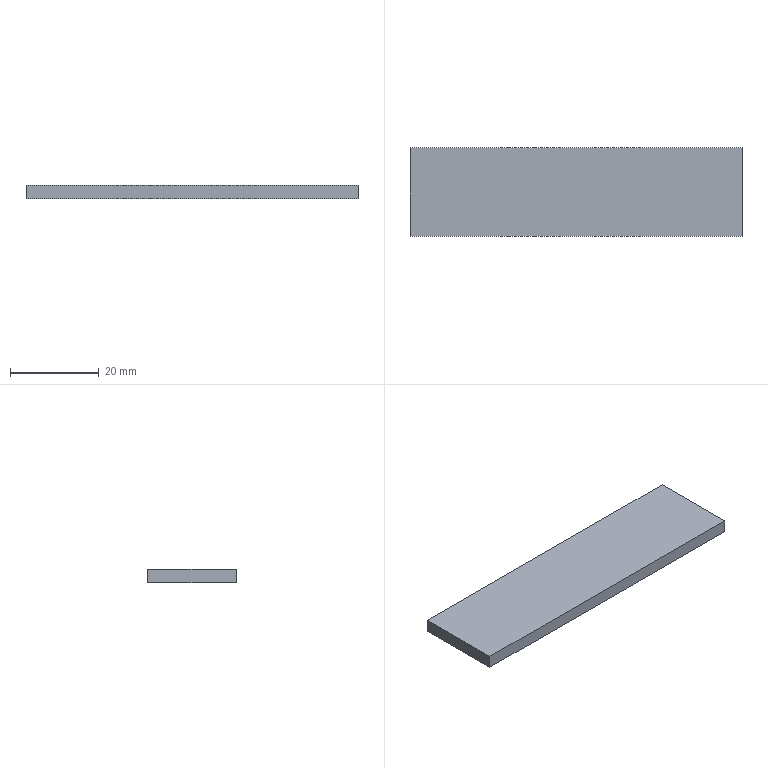Part | STEP file | 7100517 | 1 solid | 6 faces | box 75 x 20 x 3 mm | volume 4500 mm3 | plane 6
STEP:
#1=CARTESIAN_POINT('',(0.,0.,0.));
#2=DIRECTION('',(0.,0.,1.));
#3=DIRECTION('',(1.,0.,0.));
#4=AXIS2_PLACEMENT_3D('',#1,#2,#3);
#5=CARTESIAN_POINT('',(-37.5,10.,0.));
#6=VERTEX_POINT('',#5);
#7=CARTESIAN_POINT('',(-37.5,-10.,0.));
#8=VERTEX_POINT('',#7);
#9=CARTESIAN_POINT('',(-37.5,10.,0.));
#10=DIRECTION('',(0.,-1.,0.));
#11=VECTOR('',#10,1.);
#12=LINE('',#9,#11);
#13=CARTESIAN_POINT('',(-37.5,10.,3.));
#14=DIRECTION('',(1.,0.,0.));
#15=DIRECTION('',(0.,0.,-1.));
#16=AXIS2_PLACEMENT_3D('',#13,#14,#15);
#17=PLANE('',#16);
#18=CARTESIAN_POINT('',(3.,0.));
#19=DIRECTION('',(0.,-1.));
#20=VECTOR('',#19,1.);
#21=LINE('',#18,#20);
#22=(GEOMETRIC_REPRESENTATION_CONTEXT(2)PARAMETRIC_REPRESENTATION_CONTEXT()REPRESENTATION_CONTEXT('',''));
#23=DEFINITIONAL_REPRESENTATION('',(#21),#22);
#24=PCURVE('',#17,#23);
#25=CARTESIAN_POINT('',(-37.5,-10.,0.));
#26=DIRECTION('',(0.,0.,1.));
#27=DIRECTION('',(1.,0.,0.));
#28=AXIS2_PLACEMENT_3D('',#25,#26,#27);
#29=PLANE('',#28);
#30=CARTESIAN_POINT('',(0.,20.));
#31=DIRECTION('',(0.,-1.));
#32=VECTOR('',#31,1.);
#33=LINE('',#30,#32);
#34=(GEOMETRIC_REPRESENTATION_CONTEXT(2)PARAMETRIC_REPRESENTATION_CONTEXT()REPRESENTATION_CONTEXT('',''));
#35=DEFINITIONAL_REPRESENTATION('',(#33),#34);
#36=PCURVE('',#29,#35);
#37=SURFACE_CURVE('',#12,(#24,#36),.PCURVE_S1.);
#38=EDGE_CURVE('',#6,#8,#37,.T.);
#39=ORIENTED_EDGE('',*,*,#38,.T.);
#40=CARTESIAN_POINT('',(-37.5,-10.,3.));
#41=VERTEX_POINT('',#40);
#42=CARTESIAN_POINT('',(-37.5,-10.,3.));
#43=DIRECTION('',(0.,0.,-1.));
#44=VECTOR('',#43,1.);
#45=LINE('',#42,#44);
#46=CARTESIAN_POINT('',(0.,-20.));
#47=DIRECTION('',(1.,0.));
#48=VECTOR('',#47,1.);
#49=LINE('',#46,#48);
#50=(GEOMETRIC_REPRESENTATION_CONTEXT(2)PARAMETRIC_REPRESENTATION_CONTEXT()REPRESENTATION_CONTEXT('',''));
#51=DEFINITIONAL_REPRESENTATION('',(#49),#50);
#52=PCURVE('',#17,#51);
#53=CARTESIAN_POINT('',(-37.5,-10.,3.));
#54=DIRECTION('',(0.,1.,0.));
#55=DIRECTION('',(0.,0.,1.));
#56=AXIS2_PLACEMENT_3D('',#53,#54,#55);
#57=PLANE('',#56);
#58=CARTESIAN_POINT('',(0.,0.));
#59=DIRECTION('',(-1.,0.));
#60=VECTOR('',#59,1.);
#61=LINE('',#58,#60);
#62=(GEOMETRIC_REPRESENTATION_CONTEXT(2)PARAMETRIC_REPRESENTATION_CONTEXT()REPRESENTATION_CONTEXT('',''));
#63=DEFINITIONAL_REPRESENTATION('',(#61),#62);
#64=PCURVE('',#57,#63);
#65=SURFACE_CURVE('',#45,(#52,#64),.PCURVE_S1.);
#66=EDGE_CURVE('',#41,#8,#65,.T.);
#67=ORIENTED_EDGE('',*,*,#66,.F.);
#68=CARTESIAN_POINT('',(-37.5,10.,3.));
#69=VERTEX_POINT('',#68);
#70=CARTESIAN_POINT('',(-37.5,10.,3.));
#71=DIRECTION('',(0.,-1.,0.));
#72=VECTOR('',#71,1.);
#73=LINE('',#70,#72);
#74=CARTESIAN_POINT('',(0.,0.));
#75=DIRECTION('',(0.,-1.));
#76=VECTOR('',#75,1.);
#77=LINE('',#74,#76);
#78=(GEOMETRIC_REPRESENTATION_CONTEXT(2)PARAMETRIC_REPRESENTATION_CONTEXT()REPRESENTATION_CONTEXT('',''));
#79=DEFINITIONAL_REPRESENTATION('',(#77),#78);
#80=PCURVE('',#17,#79);
#81=CARTESIAN_POINT('',(-37.5,-10.,3.));
#82=DIRECTION('',(0.,0.,1.));
#83=DIRECTION('',(1.,0.,0.));
#84=AXIS2_PLACEMENT_3D('',#81,#82,#83);
#85=PLANE('',#84);
#86=CARTESIAN_POINT('',(0.,20.));
#87=DIRECTION('',(0.,-1.));
#88=VECTOR('',#87,1.);
#89=LINE('',#86,#88);
#90=(GEOMETRIC_REPRESENTATION_CONTEXT(2)PARAMETRIC_REPRESENTATION_CONTEXT()REPRESENTATION_CONTEXT('',''));
#91=DEFINITIONAL_REPRESENTATION('',(#89),#90);
#92=PCURVE('',#85,#91);
#93=SURFACE_CURVE('',#73,(#80,#92),.PCURVE_S1.);
#94=EDGE_CURVE('',#69,#41,#93,.T.);
#95=ORIENTED_EDGE('',*,*,#94,.F.);
#96=CARTESIAN_POINT('',(-37.5,10.,3.));
#97=DIRECTION('',(0.,0.,-1.));
#98=VECTOR('',#97,1.);
#99=LINE('',#96,#98);
#100=CARTESIAN_POINT('',(0.,0.));
#101=DIRECTION('',(1.,0.));
#102=VECTOR('',#101,1.);
#103=LINE('',#100,#102);
#104=(GEOMETRIC_REPRESENTATION_CONTEXT(2)PARAMETRIC_REPRESENTATION_CONTEXT()REPRESENTATION_CONTEXT('',''));
#105=DEFINITIONAL_REPRESENTATION('',(#103),#104);
#106=PCURVE('',#17,#105);
#107=CARTESIAN_POINT('',(-37.5,10.,3.));
#108=DIRECTION('',(0.,-1.,0.));
#109=DIRECTION('',(0.,0.,-1.));
#110=AXIS2_PLACEMENT_3D('',#107,#108,#109);
#111=PLANE('',#110);
#112=CARTESIAN_POINT('',(0.,0.));
#113=DIRECTION('',(1.,0.));
#114=VECTOR('',#113,1.);
#115=LINE('',#112,#114);
#116=(GEOMETRIC_REPRESENTATION_CONTEXT(2)PARAMETRIC_REPRESENTATION_CONTEXT()REPRESENTATION_CONTEXT('',''));
#117=DEFINITIONAL_REPRESENTATION('',(#115),#116);
#118=PCURVE('',#111,#117);
#119=SURFACE_CURVE('',#99,(#106,#118),.PCURVE_S1.);
#120=EDGE_CURVE('',#69,#6,#119,.T.);
#121=ORIENTED_EDGE('',*,*,#120,.T.);
#122=EDGE_LOOP('',(#39,#67,#95,#121));
#123=FACE_BOUND('',#122,.T.);
#124=ADVANCED_FACE('',(#123),#17,.F.);
#125=CARTESIAN_POINT('',(37.5,-10.,0.));
#126=VERTEX_POINT('',#125);
#127=CARTESIAN_POINT('',(-37.5,-10.,0.));
#128=DIRECTION('',(1.,0.,0.));
#129=VECTOR('',#128,1.);
#130=LINE('',#127,#129);
#131=CARTESIAN_POINT('',(-3.,0.));
#132=DIRECTION('',(0.,1.));
#133=VECTOR('',#132,1.);
#134=LINE('',#131,#133);
#135=(GEOMETRIC_REPRESENTATION_CONTEXT(2)PARAMETRIC_REPRESENTATION_CONTEXT()REPRESENTATION_CONTEXT('',''));
#136=DEFINITIONAL_REPRESENTATION('',(#134),#135);
#137=PCURVE('',#57,#136);
#138=CARTESIAN_POINT('',(0.,0.));
#139=DIRECTION('',(1.,0.));
#140=VECTOR('',#139,1.);
#141=LINE('',#138,#140);
#142=(GEOMETRIC_REPRESENTATION_CONTEXT(2)PARAMETRIC_REPRESENTATION_CONTEXT()REPRESENTATION_CONTEXT('',''));
#143=DEFINITIONAL_REPRESENTATION('',(#141),#142);
#144=PCURVE('',#29,#143);
#145=SURFACE_CURVE('',#130,(#137,#144),.PCURVE_S1.);
#146=EDGE_CURVE('',#8,#126,#145,.T.);
#147=ORIENTED_EDGE('',*,*,#146,.T.);
#148=CARTESIAN_POINT('',(37.5,-10.,3.));
#149=VERTEX_POINT('',#148);
#150=CARTESIAN_POINT('',(37.5,-10.,3.));
#151=DIRECTION('',(0.,0.,-1.));
#152=VECTOR('',#151,1.);
#153=LINE('',#150,#152);
#154=CARTESIAN_POINT('',(0.,75.));
#155=DIRECTION('',(-1.,0.));
#156=VECTOR('',#155,1.);
#157=LINE('',#154,#156);
#158=(GEOMETRIC_REPRESENTATION_CONTEXT(2)PARAMETRIC_REPRESENTATION_CONTEXT()REPRESENTATION_CONTEXT('',''));
#159=DEFINITIONAL_REPRESENTATION('',(#157),#158);
#160=PCURVE('',#57,#159);
#161=CARTESIAN_POINT('',(37.5,10.,3.));
#162=DIRECTION('',(-1.,0.,0.));
#163=DIRECTION('',(0.,0.,1.));
#164=AXIS2_PLACEMENT_3D('',#161,#162,#163);
#165=PLANE('',#164);
#166=CARTESIAN_POINT('',(0.,-20.));
#167=DIRECTION('',(-1.,0.));
#168=VECTOR('',#167,1.);
#169=LINE('',#166,#168);
#170=(GEOMETRIC_REPRESENTATION_CONTEXT(2)PARAMETRIC_REPRESENTATION_CONTEXT()REPRESENTATION_CONTEXT('',''));
#171=DEFINITIONAL_REPRESENTATION('',(#169),#170);
#172=PCURVE('',#165,#171);
#173=SURFACE_CURVE('',#153,(#160,#172),.PCURVE_S1.);
#174=EDGE_CURVE('',#149,#126,#173,.T.);
#175=ORIENTED_EDGE('',*,*,#174,.F.);
#176=CARTESIAN_POINT('',(-37.5,-10.,3.));
#177=DIRECTION('',(1.,0.,0.));
#178=VECTOR('',#177,1.);
#179=LINE('',#176,#178);
#180=CARTESIAN_POINT('',(0.,0.));
#181=DIRECTION('',(0.,1.));
#182=VECTOR('',#181,1.);
#183=LINE('',#180,#182);
#184=(GEOMETRIC_REPRESENTATION_CONTEXT(2)PARAMETRIC_REPRESENTATION_CONTEXT()REPRESENTATION_CONTEXT('',''));
#185=DEFINITIONAL_REPRESENTATION('',(#183),#184);
#186=PCURVE('',#57,#185);
#187=CARTESIAN_POINT('',(0.,0.));
#188=DIRECTION('',(1.,0.));
#189=VECTOR('',#188,1.);
#190=LINE('',#187,#189);
#191=(GEOMETRIC_REPRESENTATION_CONTEXT(2)PARAMETRIC_REPRESENTATION_CONTEXT()REPRESENTATION_CONTEXT('',''));
#192=DEFINITIONAL_REPRESENTATION('',(#190),#191);
#193=PCURVE('',#85,#192);
#194=SURFACE_CURVE('',#179,(#186,#193),.PCURVE_S1.);
#195=EDGE_CURVE('',#41,#149,#194,.T.);
#196=ORIENTED_EDGE('',*,*,#195,.F.);
#197=ORIENTED_EDGE('',*,*,#66,.T.);
#198=EDGE_LOOP('',(#147,#175,#196,#197));
#199=FACE_BOUND('',#198,.T.);
#200=ADVANCED_FACE('',(#199),#57,.F.);
#201=CARTESIAN_POINT('',(37.5,10.,0.));
#202=VERTEX_POINT('',#201);
#203=CARTESIAN_POINT('',(37.5,10.,0.));
#204=DIRECTION('',(0.,1.,0.));
#205=VECTOR('',#204,1.);
#206=LINE('',#203,#205);
#207=CARTESIAN_POINT('',(-3.,0.));
#208=DIRECTION('',(0.,1.));
#209=VECTOR('',#208,1.);
#210=LINE('',#207,#209);
#211=(GEOMETRIC_REPRESENTATION_CONTEXT(2)PARAMETRIC_REPRESENTATION_CONTEXT()REPRESENTATION_CONTEXT('',''));
#212=DEFINITIONAL_REPRESENTATION('',(#210),#211);
#213=PCURVE('',#165,#212);
#214=CARTESIAN_POINT('',(75.,20.));
#215=DIRECTION('',(0.,1.));
#216=VECTOR('',#215,1.);
#217=LINE('',#214,#216);
#218=(GEOMETRIC_REPRESENTATION_CONTEXT(2)PARAMETRIC_REPRESENTATION_CONTEXT()REPRESENTATION_CONTEXT('',''));
#219=DEFINITIONAL_REPRESENTATION('',(#217),#218);
#220=PCURVE('',#29,#219);
#221=SURFACE_CURVE('',#206,(#213,#220),.PCURVE_S1.);
#222=EDGE_CURVE('',#126,#202,#221,.T.);
#223=ORIENTED_EDGE('',*,*,#222,.T.);
#224=CARTESIAN_POINT('',(37.5,10.,3.));
#225=VERTEX_POINT('',#224);
#226=CARTESIAN_POINT('',(37.5,10.,3.));
#227=DIRECTION('',(0.,0.,-1.));
#228=VECTOR('',#227,1.);
#229=LINE('',#226,#228);
#230=CARTESIAN_POINT('',(0.,0.));
#231=DIRECTION('',(-1.,0.));
#232=VECTOR('',#231,1.);
#233=LINE('',#230,#232);
#234=(GEOMETRIC_REPRESENTATION_CONTEXT(2)PARAMETRIC_REPRESENTATION_CONTEXT()REPRESENTATION_CONTEXT('',''));
#235=DEFINITIONAL_REPRESENTATION('',(#233),#234);
#236=PCURVE('',#165,#235);
#237=CARTESIAN_POINT('',(0.,75.));
#238=DIRECTION('',(1.,0.));
#239=VECTOR('',#238,1.);
#240=LINE('',#237,#239);
#241=(GEOMETRIC_REPRESENTATION_CONTEXT(2)PARAMETRIC_REPRESENTATION_CONTEXT()REPRESENTATION_CONTEXT('',''));
#242=DEFINITIONAL_REPRESENTATION('',(#240),#241);
#243=PCURVE('',#111,#242);
#244=SURFACE_CURVE('',#229,(#236,#243),.PCURVE_S1.);
#245=EDGE_CURVE('',#225,#202,#244,.T.);
#246=ORIENTED_EDGE('',*,*,#245,.F.);
#247=CARTESIAN_POINT('',(37.5,10.,3.));
#248=DIRECTION('',(0.,1.,0.));
#249=VECTOR('',#248,1.);
#250=LINE('',#247,#249);
#251=CARTESIAN_POINT('',(0.,0.));
#252=DIRECTION('',(0.,1.));
#253=VECTOR('',#252,1.);
#254=LINE('',#251,#253);
#255=(GEOMETRIC_REPRESENTATION_CONTEXT(2)PARAMETRIC_REPRESENTATION_CONTEXT()REPRESENTATION_CONTEXT('',''));
#256=DEFINITIONAL_REPRESENTATION('',(#254),#255);
#257=PCURVE('',#165,#256);
#258=CARTESIAN_POINT('',(75.,20.));
#259=DIRECTION('',(0.,1.));
#260=VECTOR('',#259,1.);
#261=LINE('',#258,#260);
#262=(GEOMETRIC_REPRESENTATION_CONTEXT(2)PARAMETRIC_REPRESENTATION_CONTEXT()REPRESENTATION_CONTEXT('',''));
#263=DEFINITIONAL_REPRESENTATION('',(#261),#262);
#264=PCURVE('',#85,#263);
#265=SURFACE_CURVE('',#250,(#257,#264),.PCURVE_S1.);
#266=EDGE_CURVE('',#149,#225,#265,.T.);
#267=ORIENTED_EDGE('',*,*,#266,.F.);
#268=ORIENTED_EDGE('',*,*,#174,.T.);
#269=EDGE_LOOP('',(#223,#246,#267,#268));
#270=FACE_BOUND('',#269,.T.);
#271=ADVANCED_FACE('',(#270),#165,.F.);
#272=CARTESIAN_POINT('',(-37.5,10.,0.));
#273=DIRECTION('',(-1.,0.,0.));
#274=VECTOR('',#273,1.);
#275=LINE('',#272,#274);
#276=CARTESIAN_POINT('',(3.,0.));
#277=DIRECTION('',(0.,-1.));
#278=VECTOR('',#277,1.);
#279=LINE('',#276,#278);
#280=(GEOMETRIC_REPRESENTATION_CONTEXT(2)PARAMETRIC_REPRESENTATION_CONTEXT()REPRESENTATION_CONTEXT('',''));
#281=DEFINITIONAL_REPRESENTATION('',(#279),#280);
#282=PCURVE('',#111,#281);
#283=CARTESIAN_POINT('',(0.,20.));
#284=DIRECTION('',(-1.,0.));
#285=VECTOR('',#284,1.);
#286=LINE('',#283,#285);
#287=(GEOMETRIC_REPRESENTATION_CONTEXT(2)PARAMETRIC_REPRESENTATION_CONTEXT()REPRESENTATION_CONTEXT('',''));
#288=DEFINITIONAL_REPRESENTATION('',(#286),#287);
#289=PCURVE('',#29,#288);
#290=SURFACE_CURVE('',#275,(#282,#289),.PCURVE_S1.);
#291=EDGE_CURVE('',#202,#6,#290,.T.);
#292=ORIENTED_EDGE('',*,*,#291,.T.);
#293=ORIENTED_EDGE('',*,*,#120,.F.);
#294=CARTESIAN_POINT('',(-37.5,10.,3.));
#295=DIRECTION('',(-1.,0.,0.));
#296=VECTOR('',#295,1.);
#297=LINE('',#294,#296);
#298=CARTESIAN_POINT('',(0.,0.));
#299=DIRECTION('',(0.,-1.));
#300=VECTOR('',#299,1.);
#301=LINE('',#298,#300);
#302=(GEOMETRIC_REPRESENTATION_CONTEXT(2)PARAMETRIC_REPRESENTATION_CONTEXT()REPRESENTATION_CONTEXT('',''));
#303=DEFINITIONAL_REPRESENTATION('',(#301),#302);
#304=PCURVE('',#111,#303);
#305=CARTESIAN_POINT('',(0.,20.));
#306=DIRECTION('',(-1.,0.));
#307=VECTOR('',#306,1.);
#308=LINE('',#305,#307);
#309=(GEOMETRIC_REPRESENTATION_CONTEXT(2)PARAMETRIC_REPRESENTATION_CONTEXT()REPRESENTATION_CONTEXT('',''));
#310=DEFINITIONAL_REPRESENTATION('',(#308),#309);
#311=PCURVE('',#85,#310);
#312=SURFACE_CURVE('',#297,(#304,#311),.PCURVE_S1.);
#313=EDGE_CURVE('',#225,#69,#312,.T.);
#314=ORIENTED_EDGE('',*,*,#313,.F.);
#315=ORIENTED_EDGE('',*,*,#245,.T.);
#316=EDGE_LOOP('',(#292,#293,#314,#315));
#317=FACE_BOUND('',#316,.T.);
#318=ADVANCED_FACE('',(#317),#111,.F.);
#319=ORIENTED_EDGE('',*,*,#94,.T.);
#320=ORIENTED_EDGE('',*,*,#195,.T.);
#321=ORIENTED_EDGE('',*,*,#266,.T.);
#322=ORIENTED_EDGE('',*,*,#313,.T.);
#323=EDGE_LOOP('',(#319,#320,#321,#322));
#324=FACE_BOUND('',#323,.T.);
#325=ADVANCED_FACE('',(#324),#85,.T.);
#326=ORIENTED_EDGE('',*,*,#38,.F.);
#327=ORIENTED_EDGE('',*,*,#291,.F.);
#328=ORIENTED_EDGE('',*,*,#222,.F.);
#329=ORIENTED_EDGE('',*,*,#146,.F.);
#330=EDGE_LOOP('',(#326,#327,#328,#329));
#331=FACE_BOUND('',#330,.T.);
#332=ADVANCED_FACE('',(#331),#29,.F.);
#333=CLOSED_SHELL('',(#124,#200,#271,#318,#325,#332));
#334=MANIFOLD_SOLID_BREP('',#333);
#335=(LENGTH_UNIT()NAMED_UNIT(*)SI_UNIT(.MILLI.,.METRE.));
#336=UNCERTAINTY_MEASURE_WITH_UNIT(LENGTH_MEASURE(0.0000001),#335,'','');
#337=(NAMED_UNIT(*)PLANE_ANGLE_UNIT()SI_UNIT($,.RADIAN.));
#338=(NAMED_UNIT(*)SI_UNIT($,.STERADIAN.)SOLID_ANGLE_UNIT());
#339=(GEOMETRIC_REPRESENTATION_CONTEXT(3)GLOBAL_UNCERTAINTY_ASSIGNED_CONTEXT((#336))GLOBAL_UNIT_ASSIGNED_CONTEXT((#335,#337,#338))REPRESENTATION_CONTEXT('',''));
#340=ADVANCED_BREP_SHAPE_REPRESENTATION('',(#4,#334),#339);